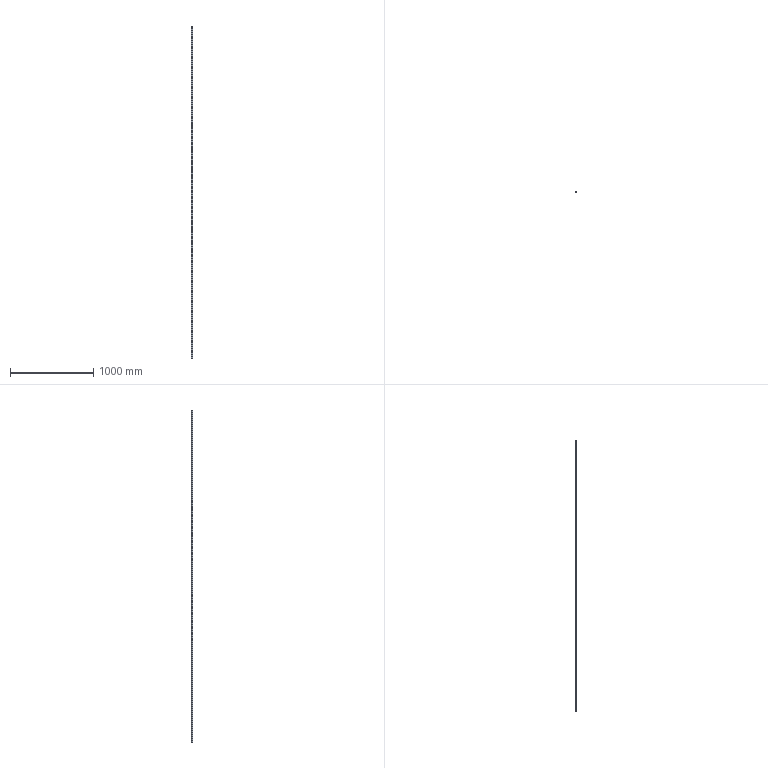Part | SolidWorks | features BaseBody 1 | 1 solid | 361 faces | box 15 x 12.5 x 4000 mm | volume 674573 mm3 | cylinder 274 | plane 87 | commonest cylinder face diameters 4.5 x134 7.5 x134 1.115 x6